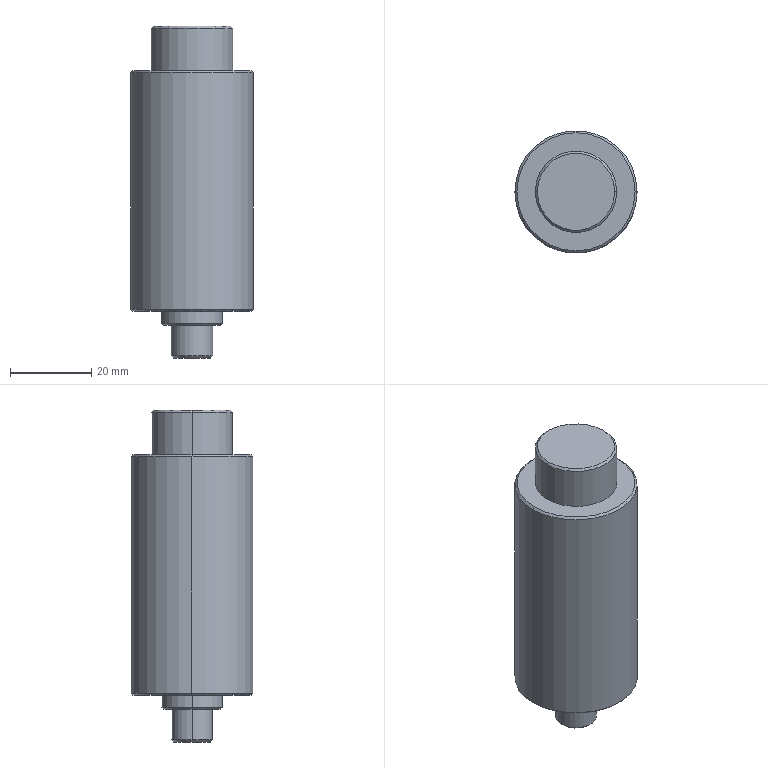Part | SolidWorks | features Chamfer 1, Revolution 1 | 1 solid | 23 faces | box 30 x 30 x 81.5 mm | volume 46379 mm3 | cone 10 | cylinder 8 | plane 5 | commonest cylinder face diameters 10.1 x2 15 x2 20 x2 30 x2
STEP:
#1=CARTESIAN_POINT('',(9.5,0.,0.));
#2=VERTEX_POINT('',#1);
#3=CARTESIAN_POINT('',(-9.5,0.,0.));
#4=VERTEX_POINT('',#3);
#5=CARTESIAN_POINT('',(0.,0.,0.));
#6=DIRECTION('',(0.,0.,1.));
#7=DIRECTION('',(-1.,0.,0.));
#8=AXIS2_PLACEMENT_3D('',#5,#6,#7);
#9=CIRCLE('',#8,9.5);
#10=EDGE_CURVE('',#2,#4,#9,.T.);
#11=ORIENTED_EDGE('',*,*,#10,.F.);
#12=CARTESIAN_POINT('',(10.,0.,-0.5));
#13=VERTEX_POINT('',#12);
#14=CARTESIAN_POINT('',(9.5,0.,0.));
#15=DIRECTION('',(0.7071,0.,-0.7071));
#16=VECTOR('',#15,1000.);
#17=LINE('',#14,#16);
#18=EDGE_CURVE('',#2,#13,#17,.T.);
#19=ORIENTED_EDGE('',*,*,#18,.T.);
#20=CARTESIAN_POINT('',(-10.,0.,-0.5));
#21=VERTEX_POINT('',#20);
#22=CARTESIAN_POINT('',(0.,0.,-0.5));
#23=DIRECTION('',(0.,0.,-1.));
#24=DIRECTION('',(-1.,0.,0.));
#25=AXIS2_PLACEMENT_3D('',#22,#23,#24);
#26=CIRCLE('',#25,10.);
#27=EDGE_CURVE('',#21,#13,#26,.T.);
#28=ORIENTED_EDGE('',*,*,#27,.F.);
#29=CARTESIAN_POINT('',(-9.5,0.,0.));
#30=DIRECTION('',(-0.7071,0.,-0.7071));
#31=VECTOR('',#30,1000.);
#32=LINE('',#29,#31);
#33=EDGE_CURVE('',#4,#21,#32,.T.);
#34=ORIENTED_EDGE('',*,*,#33,.F.);
#35=EDGE_LOOP('',(#11,#19,#28,#34));
#36=FACE_OUTER_BOUND('',#35,.T.);
#37=CARTESIAN_POINT('',(0.,0.,0.));
#38=DIRECTION('',(0.,0.,-1.));
#39=DIRECTION('',(-1.,0.,0.));
#40=AXIS2_PLACEMENT_3D('',#37,#38,#39);
#41=CONICAL_SURFACE('',#40,9.5,0.7854);
#42=ADVANCED_FACE('',(#36),#41,.T.);
#43=CARTESIAN_POINT('',(14.5,0.,-11.));
#44=VERTEX_POINT('',#43);
#45=CARTESIAN_POINT('',(-14.5,0.,-11.));
#46=VERTEX_POINT('',#45);
#47=CARTESIAN_POINT('',(0.,0.,-11.));
#48=DIRECTION('',(0.,0.,1.));
#49=DIRECTION('',(-1.,0.,0.));
#50=AXIS2_PLACEMENT_3D('',#47,#48,#49);
#51=CIRCLE('',#50,14.5);
#52=EDGE_CURVE('',#44,#46,#51,.T.);
#53=ORIENTED_EDGE('',*,*,#52,.F.);
#54=CARTESIAN_POINT('',(15.,0.,-11.5));
#55=VERTEX_POINT('',#54);
#56=CARTESIAN_POINT('',(14.5,0.,-11.));
#57=DIRECTION('',(0.7071,0.,-0.7071));
#58=VECTOR('',#57,1000.);
#59=LINE('',#56,#58);
#60=EDGE_CURVE('',#44,#55,#59,.T.);
#61=ORIENTED_EDGE('',*,*,#60,.T.);
#62=CARTESIAN_POINT('',(-15.,0.,-11.5));
#63=VERTEX_POINT('',#62);
#64=CARTESIAN_POINT('',(0.,0.,-11.5));
#65=DIRECTION('',(0.,0.,-1.));
#66=DIRECTION('',(-1.,0.,0.));
#67=AXIS2_PLACEMENT_3D('',#64,#65,#66);
#68=CIRCLE('',#67,15.);
#69=EDGE_CURVE('',#63,#55,#68,.T.);
#70=ORIENTED_EDGE('',*,*,#69,.F.);
#71=CARTESIAN_POINT('',(-14.5,0.,-11.));
#72=DIRECTION('',(-0.7071,0.,-0.7071));
#73=VECTOR('',#72,1000.);
#74=LINE('',#71,#73);
#75=EDGE_CURVE('',#46,#63,#74,.T.);
#76=ORIENTED_EDGE('',*,*,#75,.F.);
#77=EDGE_LOOP('',(#53,#61,#70,#76));
#78=FACE_OUTER_BOUND('',#77,.T.);
#79=CARTESIAN_POINT('',(0.,0.,-11.));
#80=DIRECTION('',(0.,0.,-1.));
#81=DIRECTION('',(-1.,0.,0.));
#82=AXIS2_PLACEMENT_3D('',#79,#80,#81);
#83=CONICAL_SURFACE('',#82,14.5,0.7854);
#84=ADVANCED_FACE('',(#78),#83,.T.);
#85=CARTESIAN_POINT('',(-14.5,0.,-70.));
#86=VERTEX_POINT('',#85);
#87=CARTESIAN_POINT('',(14.5,0.,-70.));
#88=VERTEX_POINT('',#87);
#89=CARTESIAN_POINT('',(0.,0.,-70.));
#90=DIRECTION('',(0.,0.,-1.));
#91=DIRECTION('',(1.,0.,0.));
#92=AXIS2_PLACEMENT_3D('',#89,#90,#91);
#93=CIRCLE('',#92,14.5);
#94=EDGE_CURVE('',#86,#88,#93,.T.);
#95=ORIENTED_EDGE('',*,*,#94,.F.);
#96=CARTESIAN_POINT('',(-15.,0.,-69.5));
#97=VERTEX_POINT('',#96);
#98=CARTESIAN_POINT('',(-15.,0.,-69.5));
#99=DIRECTION('',(-0.7071,0.,0.7071));
#100=VECTOR('',#99,1000.);
#101=LINE('',#98,#100);
#102=EDGE_CURVE('',#86,#97,#101,.T.);
#103=ORIENTED_EDGE('',*,*,#102,.T.);
#104=CARTESIAN_POINT('',(15.,0.,-69.5));
#105=VERTEX_POINT('',#104);
#106=CARTESIAN_POINT('',(0.,0.,-69.5));
#107=DIRECTION('',(0.,0.,1.));
#108=DIRECTION('',(1.,0.,0.));
#109=AXIS2_PLACEMENT_3D('',#106,#107,#108);
#110=CIRCLE('',#109,15.);
#111=EDGE_CURVE('',#105,#97,#110,.T.);
#112=ORIENTED_EDGE('',*,*,#111,.F.);
#113=CARTESIAN_POINT('',(15.,0.,-69.5));
#114=DIRECTION('',(0.7071,0.,0.7071));
#115=VECTOR('',#114,1000.);
#116=LINE('',#113,#115);
#117=EDGE_CURVE('',#88,#105,#116,.T.);
#118=ORIENTED_EDGE('',*,*,#117,.F.);
#119=EDGE_LOOP('',(#95,#103,#112,#118));
#120=FACE_OUTER_BOUND('',#119,.T.);
#121=CARTESIAN_POINT('',(0.,0.,-69.5));
#122=DIRECTION('',(0.,0.,1.));
#123=DIRECTION('',(1.,0.,0.));
#124=AXIS2_PLACEMENT_3D('',#121,#122,#123);
#125=CONICAL_SURFACE('',#124,15.,0.7854);
#126=ADVANCED_FACE('',(#120),#125,.T.);
#127=CARTESIAN_POINT('',(-7.,0.,-73.5));
#128=VERTEX_POINT('',#127);
#129=CARTESIAN_POINT('',(7.,0.,-73.5));
#130=VERTEX_POINT('',#129);
#131=CARTESIAN_POINT('',(0.,0.,-73.5));
#132=DIRECTION('',(0.,0.,-1.));
#133=DIRECTION('',(1.,0.,0.));
#134=AXIS2_PLACEMENT_3D('',#131,#132,#133);
#135=CIRCLE('',#134,7.);
#136=EDGE_CURVE('',#128,#130,#135,.T.);
#137=ORIENTED_EDGE('',*,*,#136,.F.);
#138=CARTESIAN_POINT('',(-7.5,0.,-73.));
#139=VERTEX_POINT('',#138);
#140=CARTESIAN_POINT('',(-7.5,0.,-73.));
#141=DIRECTION('',(-0.7071,0.,0.7071));
#142=VECTOR('',#141,1000.);
#143=LINE('',#140,#142);
#144=EDGE_CURVE('',#128,#139,#143,.T.);
#145=ORIENTED_EDGE('',*,*,#144,.T.);
#146=CARTESIAN_POINT('',(7.5,0.,-73.));
#147=VERTEX_POINT('',#146);
#148=CARTESIAN_POINT('',(0.,0.,-73.));
#149=DIRECTION('',(0.,0.,1.));
#150=DIRECTION('',(1.,0.,0.));
#151=AXIS2_PLACEMENT_3D('',#148,#149,#150);
#152=CIRCLE('',#151,7.5);
#153=EDGE_CURVE('',#147,#139,#152,.T.);
#154=ORIENTED_EDGE('',*,*,#153,.F.);
#155=CARTESIAN_POINT('',(7.5,0.,-73.));
#156=DIRECTION('',(0.7071,0.,0.7071));
#157=VECTOR('',#156,1000.);
#158=LINE('',#155,#157);
#159=EDGE_CURVE('',#130,#147,#158,.T.);
#160=ORIENTED_EDGE('',*,*,#159,.F.);
#161=EDGE_LOOP('',(#137,#145,#154,#160));
#162=FACE_OUTER_BOUND('',#161,.T.);
#163=CARTESIAN_POINT('',(0.,0.,-73.));
#164=DIRECTION('',(0.,0.,1.));
#165=DIRECTION('',(1.,0.,0.));
#166=AXIS2_PLACEMENT_3D('',#163,#164,#165);
#167=CONICAL_SURFACE('',#166,7.5,0.7854);
#168=ADVANCED_FACE('',(#162),#167,.T.);
#169=CARTESIAN_POINT('',(-4.55,0.,-81.5));
#170=VERTEX_POINT('',#169);
#171=CARTESIAN_POINT('',(4.55,0.,-81.5));
#172=VERTEX_POINT('',#171);
#173=CARTESIAN_POINT('',(0.,0.,-81.5));
#174=DIRECTION('',(0.,0.,-1.));
#175=DIRECTION('',(1.,0.,0.));
#176=AXIS2_PLACEMENT_3D('',#173,#174,#175);
#177=CIRCLE('',#176,4.55);
#178=EDGE_CURVE('',#170,#172,#177,.T.);
#179=ORIENTED_EDGE('',*,*,#178,.F.);
#180=CARTESIAN_POINT('',(-5.05,0.,-81.));
#181=VERTEX_POINT('',#180);
#182=CARTESIAN_POINT('',(-5.05,0.,-81.));
#183=DIRECTION('',(-0.7071,0.,0.7071));
#184=VECTOR('',#183,1000.);
#185=LINE('',#182,#184);
#186=EDGE_CURVE('',#170,#181,#185,.T.);
#187=ORIENTED_EDGE('',*,*,#186,.T.);
#188=CARTESIAN_POINT('',(5.05,0.,-81.));
#189=VERTEX_POINT('',#188);
#190=CARTESIAN_POINT('',(0.,0.,-81.));
#191=DIRECTION('',(0.,0.,1.));
#192=DIRECTION('',(1.,0.,0.));
#193=AXIS2_PLACEMENT_3D('',#190,#191,#192);
#194=CIRCLE('',#193,5.05);
#195=EDGE_CURVE('',#189,#181,#194,.T.);
#196=ORIENTED_EDGE('',*,*,#195,.F.);
#197=CARTESIAN_POINT('',(5.05,0.,-81.));
#198=DIRECTION('',(0.7071,0.,0.7071));
#199=VECTOR('',#198,1000.);
#200=LINE('',#197,#199);
#201=EDGE_CURVE('',#172,#189,#200,.T.);
#202=ORIENTED_EDGE('',*,*,#201,.F.);
#203=EDGE_LOOP('',(#179,#187,#196,#202));
#204=FACE_OUTER_BOUND('',#203,.T.);
#205=CARTESIAN_POINT('',(0.,0.,-81.));
#206=DIRECTION('',(0.,0.,1.));
#207=DIRECTION('',(1.,0.,0.));
#208=AXIS2_PLACEMENT_3D('',#205,#206,#207);
#209=CONICAL_SURFACE('',#208,5.05,0.7854);
#210=ADVANCED_FACE('',(#204),#209,.T.);
#211=CARTESIAN_POINT('',(10.,0.,-11.));
#212=VERTEX_POINT('',#211);
#213=CARTESIAN_POINT('',(-10.,0.,-11.));
#214=VERTEX_POINT('',#213);
#215=CARTESIAN_POINT('',(0.,0.,-11.));
#216=DIRECTION('',(0.,0.,1.));
#217=DIRECTION('',(1.,0.,0.));
#218=AXIS2_PLACEMENT_3D('',#215,#216,#217);
#219=CIRCLE('',#218,10.);
#220=EDGE_CURVE('',#212,#214,#219,.T.);
#221=ORIENTED_EDGE('',*,*,#220,.T.);
#222=CARTESIAN_POINT('',(-10.,0.,0.));
#223=DIRECTION('',(0.,0.,1.));
#224=VECTOR('',#223,1000.);
#225=LINE('',#222,#224);
#226=EDGE_CURVE('',#214,#21,#225,.T.);
#227=ORIENTED_EDGE('',*,*,#226,.T.);
#228=ORIENTED_EDGE('',*,*,#27,.T.);
#229=CARTESIAN_POINT('',(10.,0.,0.));
#230=DIRECTION('',(0.,0.,1.));
#231=VECTOR('',#230,1000.);
#232=LINE('',#229,#231);
#233=EDGE_CURVE('',#212,#13,#232,.T.);
#234=ORIENTED_EDGE('',*,*,#233,.F.);
#235=EDGE_LOOP('',(#221,#227,#228,#234));
#236=FACE_OUTER_BOUND('',#235,.T.);
#237=CARTESIAN_POINT('',(0.,0.,0.));
#238=DIRECTION('',(0.,0.,1.));
#239=DIRECTION('',(1.,0.,0.));
#240=AXIS2_PLACEMENT_3D('',#237,#238,#239);
#241=CYLINDRICAL_SURFACE('',#240,10.);
#242=ADVANCED_FACE('',(#236),#241,.T.);
#243=ORIENTED_EDGE('',*,*,#111,.T.);
#244=CARTESIAN_POINT('',(-15.,0.,0.));
#245=DIRECTION('',(0.,0.,1.));
#246=VECTOR('',#245,1000.);
#247=LINE('',#244,#246);
#248=EDGE_CURVE('',#97,#63,#247,.T.);
#249=ORIENTED_EDGE('',*,*,#248,.T.);
#250=ORIENTED_EDGE('',*,*,#69,.T.);
#251=CARTESIAN_POINT('',(15.,0.,0.));
#252=DIRECTION('',(0.,0.,1.));
#253=VECTOR('',#252,1000.);
#254=LINE('',#251,#253);
#255=EDGE_CURVE('',#105,#55,#254,.T.);
#256=ORIENTED_EDGE('',*,*,#255,.F.);
#257=EDGE_LOOP('',(#243,#249,#250,#256));
#258=FACE_OUTER_BOUND('',#257,.T.);
#259=CARTESIAN_POINT('',(0.,0.,0.));
#260=DIRECTION('',(0.,0.,1.));
#261=DIRECTION('',(1.,0.,0.));
#262=AXIS2_PLACEMENT_3D('',#259,#260,#261);
#263=CYLINDRICAL_SURFACE('',#262,15.);
#264=ADVANCED_FACE('',(#258),#263,.T.);
#265=ORIENTED_EDGE('',*,*,#153,.T.);
#266=CARTESIAN_POINT('',(-7.5,0.,-70.));
#267=VERTEX_POINT('',#266);
#268=CARTESIAN_POINT('',(-7.5,0.,0.));
#269=DIRECTION('',(0.,0.,1.));
#270=VECTOR('',#269,1000.);
#271=LINE('',#268,#270);
#272=EDGE_CURVE('',#139,#267,#271,.T.);
#273=ORIENTED_EDGE('',*,*,#272,.T.);
#274=CARTESIAN_POINT('',(7.5,0.,-70.));
#275=VERTEX_POINT('',#274);
#276=CARTESIAN_POINT('',(0.,0.,-70.));
#277=DIRECTION('',(0.,0.,1.));
#278=DIRECTION('',(1.,0.,0.));
#279=AXIS2_PLACEMENT_3D('',#276,#277,#278);
#280=CIRCLE('',#279,7.5);
#281=EDGE_CURVE('',#275,#267,#280,.T.);
#282=ORIENTED_EDGE('',*,*,#281,.F.);
#283=CARTESIAN_POINT('',(7.5,0.,0.));
#284=DIRECTION('',(0.,0.,1.));
#285=VECTOR('',#284,1000.);
#286=LINE('',#283,#285);
#287=EDGE_CURVE('',#147,#275,#286,.T.);
#288=ORIENTED_EDGE('',*,*,#287,.F.);
#289=EDGE_LOOP('',(#265,#273,#282,#288));
#290=FACE_OUTER_BOUND('',#289,.T.);
#291=CARTESIAN_POINT('',(0.,0.,0.));
#292=DIRECTION('',(0.,0.,1.));
#293=DIRECTION('',(1.,0.,0.));
#294=AXIS2_PLACEMENT_3D('',#291,#292,#293);
#295=CYLINDRICAL_SURFACE('',#294,7.5);
#296=ADVANCED_FACE('',(#290),#295,.T.);
#297=ORIENTED_EDGE('',*,*,#195,.T.);
#298=CARTESIAN_POINT('',(-5.05,0.,-73.5));
#299=VERTEX_POINT('',#298);
#300=CARTESIAN_POINT('',(-5.05,0.,0.));
#301=DIRECTION('',(0.,0.,1.));
#302=VECTOR('',#301,1000.);
#303=LINE('',#300,#302);
#304=EDGE_CURVE('',#181,#299,#303,.T.);
#305=ORIENTED_EDGE('',*,*,#304,.T.);
#306=CARTESIAN_POINT('',(5.05,0.,-73.5));
#307=VERTEX_POINT('',#306);
#308=CARTESIAN_POINT('',(0.,0.,-73.5));
#309=DIRECTION('',(0.,0.,1.));
#310=DIRECTION('',(1.,0.,0.));
#311=AXIS2_PLACEMENT_3D('',#308,#309,#310);
#312=CIRCLE('',#311,5.05);
#313=EDGE_CURVE('',#307,#299,#312,.T.);
#314=ORIENTED_EDGE('',*,*,#313,.F.);
#315=CARTESIAN_POINT('',(5.05,0.,0.));
#316=DIRECTION('',(0.,0.,1.));
#317=VECTOR('',#316,1000.);
#318=LINE('',#315,#317);
#319=EDGE_CURVE('',#189,#307,#318,.T.);
#320=ORIENTED_EDGE('',*,*,#319,.F.);
#321=EDGE_LOOP('',(#297,#305,#314,#320));
#322=FACE_OUTER_BOUND('',#321,.T.);
#323=CARTESIAN_POINT('',(0.,0.,0.));
#324=DIRECTION('',(0.,0.,1.));
#325=DIRECTION('',(1.,0.,0.));
#326=AXIS2_PLACEMENT_3D('',#323,#324,#325);
#327=CYLINDRICAL_SURFACE('',#326,5.05);
#328=ADVANCED_FACE('',(#322),#327,.T.);
#329=CARTESIAN_POINT('',(0.,0.,-81.5));
#330=DIRECTION('',(0.,0.,-1.));
#331=DIRECTION('',(1.,0.,0.));
#332=AXIS2_PLACEMENT_3D('',#329,#330,#331);
#333=CIRCLE('',#332,4.55);
#334=EDGE_CURVE('',#172,#170,#333,.T.);
#335=ORIENTED_EDGE('',*,*,#334,.T.);
#336=ORIENTED_EDGE('',*,*,#178,.T.);
#337=EDGE_LOOP('',(#335,#336));
#338=FACE_OUTER_BOUND('',#337,.T.);
#339=CARTESIAN_POINT('',(0.,0.,-81.5));
#340=DIRECTION('',(0.,0.,1.));
#341=DIRECTION('',(1.,0.,0.));
#342=AXIS2_PLACEMENT_3D('',#339,#340,#341);
#343=PLANE('',#342);
#344=ADVANCED_FACE('',(#338),#343,.F.);
#345=ORIENTED_EDGE('',*,*,#304,.F.);
#346=CARTESIAN_POINT('',(0.,0.,-81.));
#347=DIRECTION('',(0.,0.,1.));
#348=DIRECTION('',(1.,0.,0.));
#349=AXIS2_PLACEMENT_3D('',#346,#347,#348);
#350=CIRCLE('',#349,5.05);
#351=EDGE_CURVE('',#181,#189,#350,.T.);
#352=ORIENTED_EDGE('',*,*,#351,.T.);
#353=ORIENTED_EDGE('',*,*,#319,.T.);
#354=CARTESIAN_POINT('',(0.,0.,-73.5));
#355=DIRECTION('',(0.,0.,1.));
#356=DIRECTION('',(1.,0.,0.));
#357=AXIS2_PLACEMENT_3D('',#354,#355,#356);
#358=CIRCLE('',#357,5.05);
#359=EDGE_CURVE('',#299,#307,#358,.T.);
#360=ORIENTED_EDGE('',*,*,#359,.F.);
#361=EDGE_LOOP('',(#345,#352,#353,#360));
#362=FACE_OUTER_BOUND('',#361,.T.);
#363=CARTESIAN_POINT('',(0.,0.,0.));
#364=DIRECTION('',(0.,0.,1.));
#365=DIRECTION('',(1.,0.,0.));
#366=AXIS2_PLACEMENT_3D('',#363,#364,#365);
#367=CYLINDRICAL_SURFACE('',#366,5.05);
#368=ADVANCED_FACE('',(#362),#367,.T.);
#369=CARTESIAN_POINT('',(0.,0.,-73.5));
#370=DIRECTION('',(0.,0.,-1.));
#371=DIRECTION('',(1.,0.,0.));
#372=AXIS2_PLACEMENT_3D('',#369,#370,#371);
#373=CIRCLE('',#372,7.);
#374=EDGE_CURVE('',#130,#128,#373,.T.);
#375=ORIENTED_EDGE('',*,*,#374,.T.);
#376=ORIENTED_EDGE('',*,*,#136,.T.);
#377=EDGE_LOOP('',(#375,#376));
#378=FACE_OUTER_BOUND('',#377,.T.);
#379=ORIENTED_EDGE('',*,*,#313,.T.);
#380=ORIENTED_EDGE('',*,*,#359,.T.);
#381=EDGE_LOOP('',(#379,#380));
#382=FACE_BOUND('',#381,.T.);
#383=CARTESIAN_POINT('',(0.,5.05,-73.5));
#384=DIRECTION('',(0.,0.,1.));
#385=DIRECTION('',(1.,0.,0.));
#386=AXIS2_PLACEMENT_3D('',#383,#384,#385);
#387=PLANE('',#386);
#388=ADVANCED_FACE('',(#378,#382),#387,.F.);
#389=ORIENTED_EDGE('',*,*,#272,.F.);
#390=CARTESIAN_POINT('',(0.,0.,-73.));
#391=DIRECTION('',(0.,0.,1.));
#392=DIRECTION('',(1.,0.,0.));
#393=AXIS2_PLACEMENT_3D('',#390,#391,#392);
#394=CIRCLE('',#393,7.5);
#395=EDGE_CURVE('',#139,#147,#394,.T.);
#396=ORIENTED_EDGE('',*,*,#395,.T.);
#397=ORIENTED_EDGE('',*,*,#287,.T.);
#398=CARTESIAN_POINT('',(0.,0.,-70.));
#399=DIRECTION('',(0.,0.,1.));
#400=DIRECTION('',(1.,0.,0.));
#401=AXIS2_PLACEMENT_3D('',#398,#399,#400);
#402=CIRCLE('',#401,7.5);
#403=EDGE_CURVE('',#267,#275,#402,.T.);
#404=ORIENTED_EDGE('',*,*,#403,.F.);
#405=EDGE_LOOP('',(#389,#396,#397,#404));
#406=FACE_OUTER_BOUND('',#405,.T.);
#407=CARTESIAN_POINT('',(0.,0.,0.));
#408=DIRECTION('',(0.,0.,1.));
#409=DIRECTION('',(1.,0.,0.));
#410=AXIS2_PLACEMENT_3D('',#407,#408,#409);
#411=CYLINDRICAL_SURFACE('',#410,7.5);
#412=ADVANCED_FACE('',(#406),#411,.T.);
#413=CARTESIAN_POINT('',(0.,0.,-70.));
#414=DIRECTION('',(0.,0.,-1.));
#415=DIRECTION('',(1.,0.,0.));
#416=AXIS2_PLACEMENT_3D('',#413,#414,#415);
#417=CIRCLE('',#416,14.5);
#418=EDGE_CURVE('',#88,#86,#417,.T.);
#419=ORIENTED_EDGE('',*,*,#418,.T.);
#420=ORIENTED_EDGE('',*,*,#94,.T.);
#421=EDGE_LOOP('',(#419,#420));
#422=FACE_OUTER_BOUND('',#421,.T.);
#423=ORIENTED_EDGE('',*,*,#281,.T.);
#424=ORIENTED_EDGE('',*,*,#403,.T.);
#425=EDGE_LOOP('',(#423,#424));
#426=FACE_BOUND('',#425,.T.);
#427=CARTESIAN_POINT('',(0.,7.5,-70.));
#428=DIRECTION('',(0.,0.,1.));
#429=DIRECTION('',(1.,0.,0.));
#430=AXIS2_PLACEMENT_3D('',#427,#428,#429);
#431=PLANE('',#430);
#432=ADVANCED_FACE('',(#422,#426),#431,.F.);
#433=ORIENTED_EDGE('',*,*,#248,.F.);
#434=CARTESIAN_POINT('',(0.,0.,-69.5));
#435=DIRECTION('',(0.,0.,1.));
#436=DIRECTION('',(1.,0.,0.));
#437=AXIS2_PLACEMENT_3D('',#434,#435,#436);
#438=CIRCLE('',#437,15.);
#439=EDGE_CURVE('',#97,#105,#438,.T.);
#440=ORIENTED_EDGE('',*,*,#439,.T.);
#441=ORIENTED_EDGE('',*,*,#255,.T.);
#442=CARTESIAN_POINT('',(0.,0.,-11.5));
#443=DIRECTION('',(0.,0.,-1.));
#444=DIRECTION('',(-1.,0.,0.));
#445=AXIS2_PLACEMENT_3D('',#442,#443,#444);
#446=CIRCLE('',#445,15.);
#447=EDGE_CURVE('',#55,#63,#446,.T.);
#448=ORIENTED_EDGE('',*,*,#447,.T.);
#449=EDGE_LOOP('',(#433,#440,#441,#448));
#450=FACE_OUTER_BOUND('',#449,.T.);
#451=CARTESIAN_POINT('',(0.,0.,0.));
#452=DIRECTION('',(0.,0.,1.));
#453=DIRECTION('',(1.,0.,0.));
#454=AXIS2_PLACEMENT_3D('',#451,#452,#453);
#455=CYLINDRICAL_SURFACE('',#454,15.);
#456=ADVANCED_FACE('',(#450),#455,.T.);
#457=CARTESIAN_POINT('',(0.,0.,-11.));
#458=DIRECTION('',(0.,0.,1.));
#459=DIRECTION('',(-1.,0.,0.));
#460=AXIS2_PLACEMENT_3D('',#457,#458,#459);
#461=CIRCLE('',#460,14.5);
#462=EDGE_CURVE('',#46,#44,#461,.T.);
#463=ORIENTED_EDGE('',*,*,#462,.T.);
#464=ORIENTED_EDGE('',*,*,#52,.T.);
#465=EDGE_LOOP('',(#463,#464));
#466=FACE_OUTER_BOUND('',#465,.T.);
#467=ORIENTED_EDGE('',*,*,#220,.F.);
#468=CARTESIAN_POINT('',(0.,0.,-11.));
#469=DIRECTION('',(0.,0.,1.));
#470=DIRECTION('',(1.,0.,0.));
#471=AXIS2_PLACEMENT_3D('',#468,#469,#470);
#472=CIRCLE('',#471,10.);
#473=EDGE_CURVE('',#214,#212,#472,.T.);
#474=ORIENTED_EDGE('',*,*,#473,.F.);
#475=EDGE_LOOP('',(#467,#474));
#476=FACE_BOUND('',#475,.T.);
#477=CARTESIAN_POINT('',(0.,15.,-11.));
#478=DIRECTION('',(0.,0.,-1.));
#479=DIRECTION('',(-1.,0.,0.));
#480=AXIS2_PLACEMENT_3D('',#477,#478,#479);
#481=PLANE('',#480);
#482=ADVANCED_FACE('',(#466,#476),#481,.F.);
#483=ORIENTED_EDGE('',*,*,#226,.F.);
#484=ORIENTED_EDGE('',*,*,#473,.T.);
#485=ORIENTED_EDGE('',*,*,#233,.T.);
#486=CARTESIAN_POINT('',(0.,0.,-0.5));
#487=DIRECTION('',(0.,0.,-1.));
#488=DIRECTION('',(-1.,0.,0.));
#489=AXIS2_PLACEMENT_3D('',#486,#487,#488);
#490=CIRCLE('',#489,10.);
#491=EDGE_CURVE('',#13,#21,#490,.T.);
#492=ORIENTED_EDGE('',*,*,#491,.T.);
#493=EDGE_LOOP('',(#483,#484,#485,#492));
#494=FACE_OUTER_BOUND('',#493,.T.);
#495=CARTESIAN_POINT('',(0.,0.,0.));
#496=DIRECTION('',(0.,0.,1.));
#497=DIRECTION('',(1.,0.,0.));
#498=AXIS2_PLACEMENT_3D('',#495,#496,#497);
#499=CYLINDRICAL_SURFACE('',#498,10.);
#500=ADVANCED_FACE('',(#494),#499,.T.);
#501=CARTESIAN_POINT('',(0.,0.,0.));
#502=DIRECTION('',(0.,0.,1.));
#503=DIRECTION('',(-1.,0.,0.));
#504=AXIS2_PLACEMENT_3D('',#501,#502,#503);
#505=CIRCLE('',#504,9.5);
#506=EDGE_CURVE('',#4,#2,#505,.T.);
#507=ORIENTED_EDGE('',*,*,#506,.T.);
#508=ORIENTED_EDGE('',*,*,#10,.T.);
#509=EDGE_LOOP('',(#507,#508));
#510=FACE_OUTER_BOUND('',#509,.T.);
#511=CARTESIAN_POINT('',(0.,10.,0.));
#512=DIRECTION('',(0.,0.,-1.));
#513=DIRECTION('',(-1.,0.,0.));
#514=AXIS2_PLACEMENT_3D('',#511,#512,#513);
#515=PLANE('',#514);
#516=ADVANCED_FACE('',(#510),#515,.F.);
#517=ORIENTED_EDGE('',*,*,#186,.F.);
#518=ORIENTED_EDGE('',*,*,#334,.F.);
#519=ORIENTED_EDGE('',*,*,#201,.T.);
#520=ORIENTED_EDGE('',*,*,#351,.F.);
#521=EDGE_LOOP('',(#517,#518,#519,#520));
#522=FACE_OUTER_BOUND('',#521,.T.);
#523=CARTESIAN_POINT('',(0.,0.,-81.));
#524=DIRECTION('',(0.,0.,1.));
#525=DIRECTION('',(1.,0.,0.));
#526=AXIS2_PLACEMENT_3D('',#523,#524,#525);
#527=CONICAL_SURFACE('',#526,5.05,0.7854);
#528=ADVANCED_FACE('',(#522),#527,.T.);
#529=ORIENTED_EDGE('',*,*,#144,.F.);
#530=ORIENTED_EDGE('',*,*,#374,.F.);
#531=ORIENTED_EDGE('',*,*,#159,.T.);
#532=ORIENTED_EDGE('',*,*,#395,.F.);
#533=EDGE_LOOP('',(#529,#530,#531,#532));
#534=FACE_OUTER_BOUND('',#533,.T.);
#535=CARTESIAN_POINT('',(0.,0.,-73.));
#536=DIRECTION('',(0.,0.,1.));
#537=DIRECTION('',(1.,0.,0.));
#538=AXIS2_PLACEMENT_3D('',#535,#536,#537);
#539=CONICAL_SURFACE('',#538,7.5,0.7854);
#540=ADVANCED_FACE('',(#534),#539,.T.);
#541=ORIENTED_EDGE('',*,*,#102,.F.);
#542=ORIENTED_EDGE('',*,*,#418,.F.);
#543=ORIENTED_EDGE('',*,*,#117,.T.);
#544=ORIENTED_EDGE('',*,*,#439,.F.);
#545=EDGE_LOOP('',(#541,#542,#543,#544));
#546=FACE_OUTER_BOUND('',#545,.T.);
#547=CARTESIAN_POINT('',(0.,0.,-69.5));
#548=DIRECTION('',(0.,0.,1.));
#549=DIRECTION('',(1.,0.,0.));
#550=AXIS2_PLACEMENT_3D('',#547,#548,#549);
#551=CONICAL_SURFACE('',#550,15.,0.7854);
#552=ADVANCED_FACE('',(#546),#551,.T.);
#553=ORIENTED_EDGE('',*,*,#60,.F.);
#554=ORIENTED_EDGE('',*,*,#462,.F.);
#555=ORIENTED_EDGE('',*,*,#75,.T.);
#556=ORIENTED_EDGE('',*,*,#447,.F.);
#557=EDGE_LOOP('',(#553,#554,#555,#556));
#558=FACE_OUTER_BOUND('',#557,.T.);
#559=CARTESIAN_POINT('',(0.,0.,-11.));
#560=DIRECTION('',(0.,0.,-1.));
#561=DIRECTION('',(-1.,0.,0.));
#562=AXIS2_PLACEMENT_3D('',#559,#560,#561);
#563=CONICAL_SURFACE('',#562,14.5,0.7854);
#564=ADVANCED_FACE('',(#558),#563,.T.);
#565=ORIENTED_EDGE('',*,*,#18,.F.);
#566=ORIENTED_EDGE('',*,*,#506,.F.);
#567=ORIENTED_EDGE('',*,*,#33,.T.);
#568=ORIENTED_EDGE('',*,*,#491,.F.);
#569=EDGE_LOOP('',(#565,#566,#567,#568));
#570=FACE_OUTER_BOUND('',#569,.T.);
#571=CARTESIAN_POINT('',(0.,0.,0.));
#572=DIRECTION('',(0.,0.,-1.));
#573=DIRECTION('',(-1.,0.,0.));
#574=AXIS2_PLACEMENT_3D('',#571,#572,#573);
#575=CONICAL_SURFACE('',#574,9.5,0.7854);
#576=ADVANCED_FACE('',(#570),#575,.T.);
#577=CLOSED_SHELL('',(#42,#84,#126,#168,#210,#242,#264,#296,#328,#344,#368,#388,#412,#432,#456,#482,#500,#516,#528,#540,#552,#564,#576));
#578=MANIFOLD_SOLID_BREP('',#577);
#579=CARTESIAN_POINT('',(0.,0.,0.));
#580=DIRECTION('',(0.,0.,1.));
#581=DIRECTION('',(1.,0.,0.));
#582=AXIS2_PLACEMENT_3D('',#579,#580,#581);
#583=(LENGTH_UNIT()NAMED_UNIT(*)SI_UNIT(.MILLI.,.METRE.));
#584=UNCERTAINTY_MEASURE_WITH_UNIT(LENGTH_MEASURE(0.00001),#583,'','');
#585=(NAMED_UNIT(*)PLANE_ANGLE_UNIT()SI_UNIT($,.RADIAN.));
#586=(NAMED_UNIT(*)SI_UNIT($,.STERADIAN.)SOLID_ANGLE_UNIT());
#587=(GEOMETRIC_REPRESENTATION_CONTEXT(3)GLOBAL_UNCERTAINTY_ASSIGNED_CONTEXT((#584))GLOBAL_UNIT_ASSIGNED_CONTEXT((#583,#585,#586))REPRESENTATION_CONTEXT('',''));
#588=ADVANCED_BREP_SHAPE_REPRESENTATION('',(#578,#582),#587);